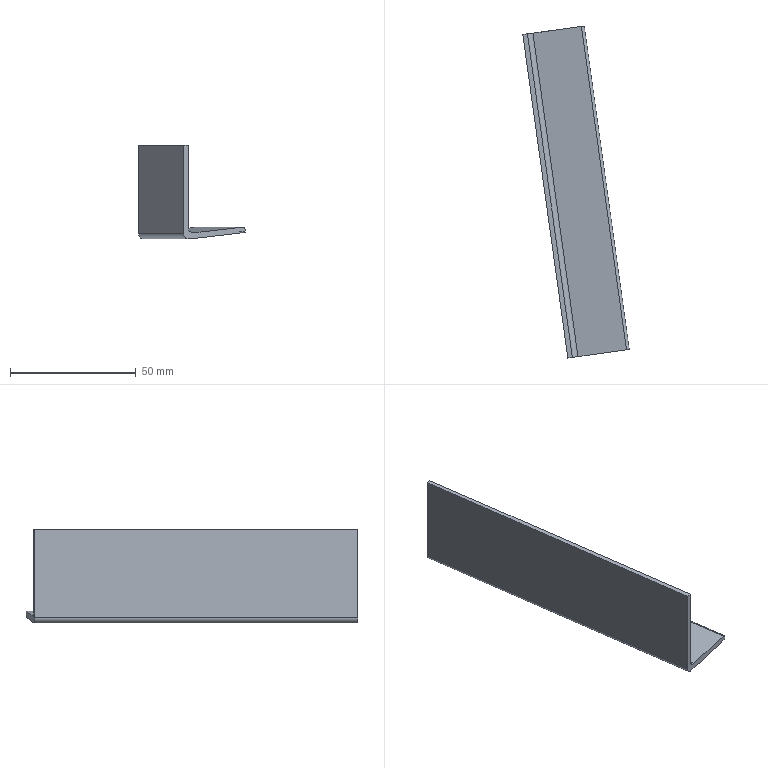Part | STEP file | 444_4 | 1 solid | 16 faces | box 42.378 x 132.163 x 37.433 mm | volume 15585 mm3 | plane 12 | cylinder 4 | commonest cylinder face diameters 4.011 x2 0.2 x1 2.007 x1
STEP:
#1=CARTESIAN_POINT('',(0.,0.,0.));
#2=DIRECTION('',(0.,0.,1.));
#3=DIRECTION('',(1.,0.,0.));
#4=AXIS2_PLACEMENT_3D('',#1,#2,#3);
#5=CARTESIAN_POINT('',(-137.211,-15.124,130.48));
#6=VERTEX_POINT('',#5);
#7=CARTESIAN_POINT('',(-119.294,-143.883,130.48));
#8=VERTEX_POINT('',#7);
#9=CARTESIAN_POINT('',(-137.211,-15.124,130.48));
#10=DIRECTION('',(0.1378,-0.9905,0.));
#11=VECTOR('',#10,1.);
#12=LINE('',#9,#11);
#13=CARTESIAN_POINT('',(-128.351,-79.517,130.48));
#14=DIRECTION('',(0.1378,-0.9905,0.));
#15=DIRECTION('',(0.9905,0.1378,0.));
#16=AXIS2_PLACEMENT_3D('',#13,#14,#15);
#17=CYLINDRICAL_SURFACE('',#16,0.09985);
#18=CARTESIAN_POINT('',(6.283,-65.));
#19=DIRECTION('',(0.,1.));
#20=VECTOR('',#19,1.);
#21=LINE('',#18,#20);
#22=(GEOMETRIC_REPRESENTATION_CONTEXT(2)PARAMETRIC_REPRESENTATION_CONTEXT()REPRESENTATION_CONTEXT('',''));
#23=DEFINITIONAL_REPRESENTATION('',(#21),#22);
#24=PCURVE('',#17,#23);
#25=CARTESIAN_POINT('',(-137.211,-15.124,131.521));
#26=DIRECTION('',(-0.9905,-0.1378,0.));
#27=DIRECTION('',(0.1378,-0.9905,0.));
#28=AXIS2_PLACEMENT_3D('',#25,#26,#27);
#29=PLANE('',#28);
#30=CARTESIAN_POINT('',(0.,-1.041));
#31=DIRECTION('',(1.,0.));
#32=VECTOR('',#31,1.);
#33=LINE('',#30,#32);
#34=(GEOMETRIC_REPRESENTATION_CONTEXT(2)PARAMETRIC_REPRESENTATION_CONTEXT()REPRESENTATION_CONTEXT('',''));
#35=DEFINITIONAL_REPRESENTATION('',(#33),#34);
#36=PCURVE('',#29,#35);
#37=SURFACE_CURVE('',#12,(#24,#36),.PCURVE_S1.);
#38=EDGE_CURVE('',#6,#8,#37,.T.);
#39=ORIENTED_EDGE('',*,*,#38,.T.);
#40=CARTESIAN_POINT('',(-119.381,-143.895,130.381));
#41=VERTEX_POINT('',#40);
#42=CARTESIAN_POINT('',(-119.392,-143.897,130.48));
#43=DIRECTION('',(-0.1378,0.9905,0.));
#44=DIRECTION('',(0.9905,0.1378,0.));
#45=AXIS2_PLACEMENT_3D('',#42,#43,#44);
#46=CIRCLE('',#45,0.09985);
#47=CARTESIAN_POINT('',(12.566,65.));
#48=DIRECTION('',(-1.,0.));
#49=VECTOR('',#48,1.);
#50=LINE('',#47,#49);
#51=(GEOMETRIC_REPRESENTATION_CONTEXT(2)PARAMETRIC_REPRESENTATION_CONTEXT()REPRESENTATION_CONTEXT('',''));
#52=DEFINITIONAL_REPRESENTATION('',(#50),#51);
#53=PCURVE('',#17,#52);
#54=CARTESIAN_POINT('',(17.376,-124.865,0.));
#55=DIRECTION('',(0.1378,-0.9905,0.));
#56=DIRECTION('',(0.9905,0.1378,0.));
#57=AXIS2_PLACEMENT_3D('',#54,#55,#56);
#58=PLANE('',#57);
#59=CARTESIAN_POINT('',(-137.986,130.48));
#60=CARTESIAN_POINT('',(-137.986,130.307));
#61=CARTESIAN_POINT('',(-138.136,130.393));
#62=CARTESIAN_POINT('',(-138.286,130.48));
#63=CARTESIAN_POINT('',(-138.136,130.566));
#64=CARTESIAN_POINT('',(-137.986,130.653));
#65=CARTESIAN_POINT('',(-137.986,130.48));
#66=(BOUNDED_CURVE()B_SPLINE_CURVE(2,(#59,#60,#61,#62,#63,#64,#65),.UNSPECIFIED.,.T.,.F.)B_SPLINE_CURVE_WITH_KNOTS((1,2,2,2,2,1),(-2.094,0.,2.094,4.189,6.283,8.378),.UNSPECIFIED.)CURVE()GEOMETRIC_REPRESENTATION_ITEM()RATIONAL_B_SPLINE_CURVE((1.,0.5,1.,0.5,1.,0.5,1.))REPRESENTATION_ITEM(''));
#67=(GEOMETRIC_REPRESENTATION_CONTEXT(2)PARAMETRIC_REPRESENTATION_CONTEXT()REPRESENTATION_CONTEXT('',''));
#68=DEFINITIONAL_REPRESENTATION('',(#66),#67);
#69=PCURVE('',#58,#68);
#70=SURFACE_CURVE('',#46,(#53,#69),.PCURVE_S1.);
#71=EDGE_CURVE('',#8,#41,#70,.T.);
#72=ORIENTED_EDGE('',*,*,#71,.T.);
#73=CARTESIAN_POINT('',(-137.299,-15.136,130.381));
#74=VERTEX_POINT('',#73);
#75=CARTESIAN_POINT('',(-119.381,-143.895,130.381));
#76=DIRECTION('',(-0.1378,0.9905,0.));
#77=VECTOR('',#76,1.);
#78=LINE('',#75,#77);
#79=CARTESIAN_POINT('',(4.827,65.));
#80=DIRECTION('',(0.,-1.));
#81=VECTOR('',#80,1.);
#82=LINE('',#79,#81);
#83=(GEOMETRIC_REPRESENTATION_CONTEXT(2)PARAMETRIC_REPRESENTATION_CONTEXT()REPRESENTATION_CONTEXT('',''));
#84=DEFINITIONAL_REPRESENTATION('',(#82),#83);
#85=PCURVE('',#17,#84);
#86=CARTESIAN_POINT('',(-137.299,-15.136,130.381));
#87=DIRECTION('',(-0.114,-0.01586,0.9934));
#88=DIRECTION('',(0.9935,0.,0.114));
#89=AXIS2_PLACEMENT_3D('',#86,#87,#88);
#90=PLANE('',#89);
#91=CARTESIAN_POINT('',(17.801,-128.775));
#92=DIRECTION('',(-0.1369,0.9906));
#93=VECTOR('',#92,1.);
#94=LINE('',#91,#93);
#95=(GEOMETRIC_REPRESENTATION_CONTEXT(2)PARAMETRIC_REPRESENTATION_CONTEXT()REPRESENTATION_CONTEXT('',''));
#96=DEFINITIONAL_REPRESENTATION('',(#94),#95);
#97=PCURVE('',#90,#96);
#98=SURFACE_CURVE('',#78,(#85,#97),.PCURVE_S1.);
#99=EDGE_CURVE('',#41,#74,#98,.T.);
#100=ORIENTED_EDGE('',*,*,#99,.T.);
#101=CARTESIAN_POINT('',(-137.31,-15.138,130.48));
#102=DIRECTION('',(0.1378,-0.9905,0.));
#103=DIRECTION('',(0.9905,0.1378,0.));
#104=AXIS2_PLACEMENT_3D('',#101,#102,#103);
#105=CIRCLE('',#104,0.09985);
#106=CARTESIAN_POINT('',(0.,-65.));
#107=DIRECTION('',(1.,0.));
#108=VECTOR('',#107,1.);
#109=LINE('',#106,#108);
#110=(GEOMETRIC_REPRESENTATION_CONTEXT(2)PARAMETRIC_REPRESENTATION_CONTEXT()REPRESENTATION_CONTEXT('',''));
#111=DEFINITIONAL_REPRESENTATION('',(#109),#110);
#112=PCURVE('',#17,#111);
#113=CARTESIAN_POINT('',(-0.5419,3.894,0.));
#114=DIRECTION('',(0.1378,-0.9905,0.));
#115=DIRECTION('',(0.9905,0.1378,0.));
#116=AXIS2_PLACEMENT_3D('',#113,#114,#115);
#117=PLANE('',#116);
#118=CARTESIAN_POINT('',(-138.086,130.48));
#119=DIRECTION('',(1.,0.));
#120=AXIS2_PLACEMENT_2D('',#118,#119);
#121=CIRCLE('',#120,0.09985);
#122=(GEOMETRIC_REPRESENTATION_CONTEXT(2)PARAMETRIC_REPRESENTATION_CONTEXT()REPRESENTATION_CONTEXT('',''));
#123=DEFINITIONAL_REPRESENTATION('',(#121),#122);
#124=PCURVE('',#117,#123);
#125=SURFACE_CURVE('',#105,(#112,#124),.PCURVE_S1.);
#126=EDGE_CURVE('',#74,#6,#125,.T.);
#127=ORIENTED_EDGE('',*,*,#126,.T.);
#128=EDGE_LOOP('',(#39,#72,#100,#127));
#129=FACE_BOUND('',#128,.T.);
#130=ADVANCED_FACE('',(#129),#17,.T.);
#131=CARTESIAN_POINT('',(-137.628,-15.182,130.342));
#132=VERTEX_POINT('',#131);
#133=CARTESIAN_POINT('',(-137.299,-15.136,130.381));
#134=DIRECTION('',(-0.9839,-0.1369,-0.1151));
#135=VECTOR('',#134,1.);
#136=LINE('',#133,#135);
#137=CARTESIAN_POINT('',(0.,0.));
#138=DIRECTION('',(-0.9906,-0.1369));
#139=VECTOR('',#138,1.);
#140=LINE('',#137,#139);
#141=(GEOMETRIC_REPRESENTATION_CONTEXT(2)PARAMETRIC_REPRESENTATION_CONTEXT()REPRESENTATION_CONTEXT('',''));
#142=DEFINITIONAL_REPRESENTATION('',(#140),#141);
#143=PCURVE('',#90,#142);
#144=CARTESIAN_POINT('',(-138.075,130.381));
#145=DIRECTION('',(-0.9934,-0.1151));
#146=VECTOR('',#145,1.);
#147=LINE('',#144,#146);
#148=(GEOMETRIC_REPRESENTATION_CONTEXT(2)PARAMETRIC_REPRESENTATION_CONTEXT()REPRESENTATION_CONTEXT('',''));
#149=DEFINITIONAL_REPRESENTATION('',(#147),#148);
#150=PCURVE('',#117,#149);
#151=SURFACE_CURVE('',#136,(#143,#150),.PCURVE_S1.);
#152=EDGE_CURVE('',#74,#132,#151,.T.);
#153=ORIENTED_EDGE('',*,*,#152,.F.);
#154=ORIENTED_EDGE('',*,*,#99,.F.);
#155=CARTESIAN_POINT('',(-119.71,-143.941,130.342));
#156=VERTEX_POINT('',#155);
#157=CARTESIAN_POINT('',(-119.71,-143.941,130.342));
#158=DIRECTION('',(0.9839,0.1369,0.1151));
#159=VECTOR('',#158,1.);
#160=LINE('',#157,#159);
#161=CARTESIAN_POINT('',(17.47,-128.821));
#162=DIRECTION('',(0.9906,0.1369));
#163=VECTOR('',#162,1.);
#164=LINE('',#161,#163);
#165=(GEOMETRIC_REPRESENTATION_CONTEXT(2)PARAMETRIC_REPRESENTATION_CONTEXT()REPRESENTATION_CONTEXT('',''));
#166=DEFINITIONAL_REPRESENTATION('',(#164),#165);
#167=PCURVE('',#90,#166);
#168=CARTESIAN_POINT('',(-138.407,130.342));
#169=DIRECTION('',(0.9934,0.1151));
#170=VECTOR('',#169,1.);
#171=LINE('',#168,#170);
#172=(GEOMETRIC_REPRESENTATION_CONTEXT(2)PARAMETRIC_REPRESENTATION_CONTEXT()REPRESENTATION_CONTEXT('',''));
#173=DEFINITIONAL_REPRESENTATION('',(#171),#172);
#174=PCURVE('',#58,#173);
#175=SURFACE_CURVE('',#160,(#167,#174),.PCURVE_S1.);
#176=EDGE_CURVE('',#156,#41,#175,.T.);
#177=ORIENTED_EDGE('',*,*,#176,.F.);
#178=CARTESIAN_POINT('',(-137.628,-15.182,130.342));
#179=DIRECTION('',(-0.1378,0.9905,0.));
#180=VECTOR('',#179,1.);
#181=LINE('',#178,#180);
#182=CARTESIAN_POINT('',(-0.3313,-0.04579));
#183=DIRECTION('',(-0.1369,0.9906));
#184=VECTOR('',#183,1.);
#185=LINE('',#182,#184);
#186=(GEOMETRIC_REPRESENTATION_CONTEXT(2)PARAMETRIC_REPRESENTATION_CONTEXT()REPRESENTATION_CONTEXT('',''));
#187=DEFINITIONAL_REPRESENTATION('',(#185),#186);
#188=PCURVE('',#90,#187);
#189=CARTESIAN_POINT('',(-137.628,-15.182,130.342));
#190=DIRECTION('',(0.9905,0.1378,-0.000000003));
#191=DIRECTION('',(-0.1378,0.9905,0.));
#192=AXIS2_PLACEMENT_3D('',#189,#190,#191);
#193=PLANE('',#192);
#194=CARTESIAN_POINT('',(0.,0.));
#195=DIRECTION('',(1.,0.));
#196=VECTOR('',#195,1.);
#197=LINE('',#194,#196);
#198=(GEOMETRIC_REPRESENTATION_CONTEXT(2)PARAMETRIC_REPRESENTATION_CONTEXT()REPRESENTATION_CONTEXT('',''));
#199=DEFINITIONAL_REPRESENTATION('',(#197),#198);
#200=PCURVE('',#193,#199);
#201=SURFACE_CURVE('',#181,(#188,#200),.PCURVE_S1.);
#202=EDGE_CURVE('',#156,#132,#201,.T.);
#203=ORIENTED_EDGE('',*,*,#202,.T.);
#204=EDGE_LOOP('',(#153,#154,#177,#203));
#205=FACE_BOUND('',#204,.T.);
#206=ADVANCED_FACE('',(#205),#90,.F.);
#207=CARTESIAN_POINT('',(-137.211,-15.124,131.521));
#208=VERTEX_POINT('',#207);
#209=CARTESIAN_POINT('',(-137.211,-15.124,131.521));
#210=DIRECTION('',(0.,0.,-1.));
#211=VECTOR('',#210,1.);
#212=LINE('',#209,#211);
#213=CARTESIAN_POINT('',(0.,0.));
#214=DIRECTION('',(0.,-1.));
#215=VECTOR('',#214,1.);
#216=LINE('',#213,#215);
#217=(GEOMETRIC_REPRESENTATION_CONTEXT(2)PARAMETRIC_REPRESENTATION_CONTEXT()REPRESENTATION_CONTEXT('',''));
#218=DEFINITIONAL_REPRESENTATION('',(#216),#217);
#219=PCURVE('',#29,#218);
#220=CARTESIAN_POINT('',(-137.986,131.521));
#221=DIRECTION('',(0.,-1.));
#222=VECTOR('',#221,1.);
#223=LINE('',#220,#222);
#224=(GEOMETRIC_REPRESENTATION_CONTEXT(2)PARAMETRIC_REPRESENTATION_CONTEXT()REPRESENTATION_CONTEXT('',''));
#225=DEFINITIONAL_REPRESENTATION('',(#223),#224);
#226=PCURVE('',#117,#225);
#227=SURFACE_CURVE('',#212,(#219,#226),.PCURVE_S1.);
#228=EDGE_CURVE('',#208,#6,#227,.T.);
#229=ORIENTED_EDGE('',*,*,#228,.F.);
#230=CARTESIAN_POINT('',(-119.294,-143.883,131.521));
#231=VERTEX_POINT('',#230);
#232=CARTESIAN_POINT('',(-128.252,-79.504,131.521));
#233=DIRECTION('',(-0.1378,0.9905,0.));
#234=VECTOR('',#233,1.);
#235=LINE('',#232,#234);
#236=CARTESIAN_POINT('',(65.,0.));
#237=DIRECTION('',(-1.,0.));
#238=VECTOR('',#237,1.);
#239=LINE('',#236,#238);
#240=(GEOMETRIC_REPRESENTATION_CONTEXT(2)PARAMETRIC_REPRESENTATION_CONTEXT()REPRESENTATION_CONTEXT('',''));
#241=DEFINITIONAL_REPRESENTATION('',(#239),#240);
#242=PCURVE('',#29,#241);
#243=CARTESIAN_POINT('',(-129.246,-79.642,131.52));
#244=DIRECTION('',(0.1378,-0.9905,0.));
#245=DIRECTION('',(0.9905,0.1378,0.));
#246=AXIS2_PLACEMENT_3D('',#243,#244,#245);
#247=CYLINDRICAL_SURFACE('',#246,1.004);
#248=CARTESIAN_POINT('',(0.0006999,0.));
#249=DIRECTION('',(0.,-1.));
#250=VECTOR('',#249,1.);
#251=LINE('',#248,#250);
#252=(GEOMETRIC_REPRESENTATION_CONTEXT(2)PARAMETRIC_REPRESENTATION_CONTEXT()REPRESENTATION_CONTEXT('',''));
#253=DEFINITIONAL_REPRESENTATION('',(#251),#252);
#254=PCURVE('',#247,#253);
#255=SURFACE_CURVE('',#235,(#242,#254),.PCURVE_S1.);
#256=EDGE_CURVE('',#231,#208,#255,.T.);
#257=ORIENTED_EDGE('',*,*,#256,.F.);
#258=CARTESIAN_POINT('',(-119.294,-143.883,131.521));
#259=DIRECTION('',(0.,0.,1.));
#260=VECTOR('',#259,1.);
#261=LINE('',#258,#260);
#262=CARTESIAN_POINT('',(130.,0.));
#263=DIRECTION('',(0.,1.));
#264=VECTOR('',#263,1.);
#265=LINE('',#262,#264);
#266=(GEOMETRIC_REPRESENTATION_CONTEXT(2)PARAMETRIC_REPRESENTATION_CONTEXT()REPRESENTATION_CONTEXT('',''));
#267=DEFINITIONAL_REPRESENTATION('',(#265),#266);
#268=PCURVE('',#29,#267);
#269=CARTESIAN_POINT('',(-137.986,131.521));
#270=DIRECTION('',(0.,1.));
#271=VECTOR('',#270,1.);
#272=LINE('',#269,#271);
#273=(GEOMETRIC_REPRESENTATION_CONTEXT(2)PARAMETRIC_REPRESENTATION_CONTEXT()REPRESENTATION_CONTEXT('',''));
#274=DEFINITIONAL_REPRESENTATION('',(#272),#273);
#275=PCURVE('',#58,#274);
#276=SURFACE_CURVE('',#261,(#268,#275),.PCURVE_S1.);
#277=EDGE_CURVE('',#8,#231,#276,.T.);
#278=ORIENTED_EDGE('',*,*,#277,.F.);
#279=ORIENTED_EDGE('',*,*,#38,.F.);
#280=EDGE_LOOP('',(#229,#257,#278,#279));
#281=FACE_BOUND('',#280,.T.);
#282=ADVANCED_FACE('',(#281),#29,.F.);
#283=CARTESIAN_POINT('',(-137.628,-15.182,130.687));
#284=VERTEX_POINT('',#283);
#285=CARTESIAN_POINT('',(-137.628,-15.182,130.342));
#286=DIRECTION('',(0.000000003,0.,1.));
#287=VECTOR('',#286,1.);
#288=LINE('',#285,#287);
#289=CARTESIAN_POINT('',(0.,0.));
#290=DIRECTION('',(0.,1.));
#291=VECTOR('',#290,1.);
#292=LINE('',#289,#291);
#293=(GEOMETRIC_REPRESENTATION_CONTEXT(2)PARAMETRIC_REPRESENTATION_CONTEXT()REPRESENTATION_CONTEXT('',''));
#294=DEFINITIONAL_REPRESENTATION('',(#292),#293);
#295=PCURVE('',#193,#294);
#296=CARTESIAN_POINT('',(-138.407,130.342));
#297=DIRECTION('',(0.000000003,1.));
#298=VECTOR('',#297,1.);
#299=LINE('',#296,#298);
#300=(GEOMETRIC_REPRESENTATION_CONTEXT(2)PARAMETRIC_REPRESENTATION_CONTEXT()REPRESENTATION_CONTEXT('',''));
#301=DEFINITIONAL_REPRESENTATION('',(#299),#300);
#302=PCURVE('',#117,#301);
#303=SURFACE_CURVE('',#288,(#295,#302),.PCURVE_S1.);
#304=EDGE_CURVE('',#132,#284,#303,.T.);
#305=ORIENTED_EDGE('',*,*,#304,.F.);
#306=ORIENTED_EDGE('',*,*,#202,.F.);
#307=CARTESIAN_POINT('',(-119.71,-143.941,130.687));
#308=VERTEX_POINT('',#307);
#309=CARTESIAN_POINT('',(-119.71,-143.941,130.342));
#310=DIRECTION('',(-0.000000003,0.,-1.));
#311=VECTOR('',#310,1.);
#312=LINE('',#309,#311);
#313=CARTESIAN_POINT('',(-130.,0.));
#314=DIRECTION('',(0.,-1.));
#315=VECTOR('',#314,1.);
#316=LINE('',#313,#315);
#317=(GEOMETRIC_REPRESENTATION_CONTEXT(2)PARAMETRIC_REPRESENTATION_CONTEXT()REPRESENTATION_CONTEXT('',''));
#318=DEFINITIONAL_REPRESENTATION('',(#316),#317);
#319=PCURVE('',#193,#318);
#320=CARTESIAN_POINT('',(-138.407,130.342));
#321=DIRECTION('',(-0.000000003,-1.));
#322=VECTOR('',#321,1.);
#323=LINE('',#320,#322);
#324=(GEOMETRIC_REPRESENTATION_CONTEXT(2)PARAMETRIC_REPRESENTATION_CONTEXT()REPRESENTATION_CONTEXT('',''));
#325=DEFINITIONAL_REPRESENTATION('',(#323),#324);
#326=PCURVE('',#58,#325);
#327=SURFACE_CURVE('',#312,(#319,#326),.PCURVE_S1.);
#328=EDGE_CURVE('',#308,#156,#327,.T.);
#329=ORIENTED_EDGE('',*,*,#328,.F.);
#330=CARTESIAN_POINT('',(-119.71,-143.941,130.687));
#331=DIRECTION('',(-0.1378,0.9905,0.));
#332=VECTOR('',#331,1.);
#333=LINE('',#330,#332);
#334=CARTESIAN_POINT('',(-130.,0.3449));
#335=DIRECTION('',(1.,0.));
#336=VECTOR('',#335,1.);
#337=LINE('',#334,#336);
#338=(GEOMETRIC_REPRESENTATION_CONTEXT(2)PARAMETRIC_REPRESENTATION_CONTEXT()REPRESENTATION_CONTEXT('',''));
#339=DEFINITIONAL_REPRESENTATION('',(#337),#338);
#340=PCURVE('',#193,#339);
#341=CARTESIAN_POINT('',(-137.628,-15.182,130.687));
#342=DIRECTION('',(0.0002938,0.00004088,1.));
#343=DIRECTION('',(1.,0.,-0.0002938));
#344=AXIS2_PLACEMENT_3D('',#341,#342,#343);
#345=PLANE('',#344);
#346=CARTESIAN_POINT('',(17.918,-128.759));
#347=DIRECTION('',(-0.1378,0.9905));
#348=VECTOR('',#347,1.);
#349=LINE('',#346,#348);
#350=(GEOMETRIC_REPRESENTATION_CONTEXT(2)PARAMETRIC_REPRESENTATION_CONTEXT()REPRESENTATION_CONTEXT('',''));
#351=DEFINITIONAL_REPRESENTATION('',(#349),#350);
#352=PCURVE('',#345,#351);
#353=SURFACE_CURVE('',#333,(#340,#352),.PCURVE_S1.);
#354=EDGE_CURVE('',#308,#284,#353,.T.);
#355=ORIENTED_EDGE('',*,*,#354,.T.);
#356=EDGE_LOOP('',(#305,#306,#329,#355));
#357=FACE_BOUND('',#356,.T.);
#358=ADVANCED_FACE('',(#357),#193,.F.);
#359=CARTESIAN_POINT('',(-138.319,-15.278,132.517));
#360=VERTEX_POINT('',#359);
#361=CARTESIAN_POINT('',(-120.402,-144.037,132.517));
#362=VERTEX_POINT('',#361);
#363=CARTESIAN_POINT('',(-138.319,-15.278,132.517));
#364=DIRECTION('',(0.1378,-0.9905,0.));
#365=VECTOR('',#364,1.);
#366=LINE('',#363,#365);
#367=CARTESIAN_POINT('',(1.686,-65.));
#368=DIRECTION('',(0.,1.));
#369=VECTOR('',#368,1.);
#370=LINE('',#367,#369);
#371=(GEOMETRIC_REPRESENTATION_CONTEXT(2)PARAMETRIC_REPRESENTATION_CONTEXT()REPRESENTATION_CONTEXT('',''));
#372=DEFINITIONAL_REPRESENTATION('',(#370),#371);
#373=PCURVE('',#247,#372);
#374=CARTESIAN_POINT('',(-157.626,-17.965,130.259));
#375=DIRECTION('',(0.114,0.01586,-0.9934));
#376=DIRECTION('',(-0.9935,0.,-0.114));
#377=AXIS2_PLACEMENT_3D('',#374,#375,#376);
#378=PLANE('',#377);
#379=CARTESIAN_POINT('',(-19.438,2.687));
#380=DIRECTION('',(-0.1369,-0.9906));
#381=VECTOR('',#380,1.);
#382=LINE('',#379,#381);
#383=(GEOMETRIC_REPRESENTATION_CONTEXT(2)PARAMETRIC_REPRESENTATION_CONTEXT()REPRESENTATION_CONTEXT('',''));
#384=DEFINITIONAL_REPRESENTATION('',(#382),#383);
#385=PCURVE('',#378,#384);
#386=SURFACE_CURVE('',#366,(#373,#385),.PCURVE_S1.);
#387=EDGE_CURVE('',#360,#362,#386,.T.);
#388=ORIENTED_EDGE('',*,*,#387,.T.);
#389=CARTESIAN_POINT('',(-120.288,-144.022,131.52));
#390=DIRECTION('',(-0.1378,0.9905,0.));
#391=DIRECTION('',(0.9905,0.1378,0.));
#392=AXIS2_PLACEMENT_3D('',#389,#390,#391);
#393=CIRCLE('',#392,1.004);
#394=CARTESIAN_POINT('',(6.283,65.));
#395=DIRECTION('',(-1.,0.));
#396=VECTOR('',#395,1.);
#397=LINE('',#394,#396);
#398=(GEOMETRIC_REPRESENTATION_CONTEXT(2)PARAMETRIC_REPRESENTATION_CONTEXT()REPRESENTATION_CONTEXT('',''));
#399=DEFINITIONAL_REPRESENTATION('',(#397),#398);
#400=PCURVE('',#247,#399);
#401=CARTESIAN_POINT('',(-137.986,131.52));
#402=CARTESIAN_POINT('',(-137.986,129.782));
#403=CARTESIAN_POINT('',(-139.492,130.651));
#404=CARTESIAN_POINT('',(-140.997,131.52));
#405=CARTESIAN_POINT('',(-139.492,132.39));
#406=CARTESIAN_POINT('',(-137.986,133.259));
#407=CARTESIAN_POINT('',(-137.986,131.52));
#408=(BOUNDED_CURVE()B_SPLINE_CURVE(2,(#401,#402,#403,#404,#405,#406,#407),.UNSPECIFIED.,.T.,.F.)B_SPLINE_CURVE_WITH_KNOTS((1,2,2,2,2,1),(-2.094,0.,2.094,4.189,6.283,8.378),.UNSPECIFIED.)CURVE()GEOMETRIC_REPRESENTATION_ITEM()RATIONAL_B_SPLINE_CURVE((1.,0.5,1.,0.5,1.,0.5,1.))REPRESENTATION_ITEM(''));
#409=(GEOMETRIC_REPRESENTATION_CONTEXT(2)PARAMETRIC_REPRESENTATION_CONTEXT()REPRESENTATION_CONTEXT('',''));
#410=DEFINITIONAL_REPRESENTATION('',(#408),#409);
#411=PCURVE('',#58,#410);
#412=SURFACE_CURVE('',#393,(#400,#411),.PCURVE_S1.);
#413=EDGE_CURVE('',#362,#231,#412,.T.);
#414=ORIENTED_EDGE('',*,*,#413,.T.);
#415=ORIENTED_EDGE('',*,*,#256,.T.);
#416=CARTESIAN_POINT('',(-138.205,-15.262,131.52));
#417=DIRECTION('',(0.1378,-0.9905,0.));
#418=DIRECTION('',(0.9905,0.1378,0.));
#419=AXIS2_PLACEMENT_3D('',#416,#417,#418);
#420=CIRCLE('',#419,1.004);
#421=CARTESIAN_POINT('',(0.,-65.));
#422=DIRECTION('',(1.,0.));
#423=VECTOR('',#422,1.);
#424=LINE('',#421,#423);
#425=(GEOMETRIC_REPRESENTATION_CONTEXT(2)PARAMETRIC_REPRESENTATION_CONTEXT()REPRESENTATION_CONTEXT('',''));
#426=DEFINITIONAL_REPRESENTATION('',(#424),#425);
#427=PCURVE('',#247,#426);
#428=CARTESIAN_POINT('',(-138.99,131.52));
#429=DIRECTION('',(1.,0.));
#430=AXIS2_PLACEMENT_2D('',#428,#429);
#431=CIRCLE('',#430,1.004);
#432=(GEOMETRIC_REPRESENTATION_CONTEXT(2)PARAMETRIC_REPRESENTATION_CONTEXT()REPRESENTATION_CONTEXT('',''));
#433=DEFINITIONAL_REPRESENTATION('',(#431),#432);
#434=PCURVE('',#117,#433);
#435=SURFACE_CURVE('',#420,(#427,#434),.PCURVE_S1.);
#436=EDGE_CURVE('',#208,#360,#435,.T.);
#437=ORIENTED_EDGE('',*,*,#436,.T.);
#438=EDGE_LOOP('',(#388,#414,#415,#437));
#439=FACE_BOUND('',#438,.T.);
#440=ADVANCED_FACE('',(#439),#247,.T.);
#441=CARTESIAN_POINT('',(-139.46,-15.437,130.688));
#442=VERTEX_POINT('',#441);
#443=CARTESIAN_POINT('',(-139.46,-15.437,130.128));
#444=VERTEX_POINT('',#443);
#445=CARTESIAN_POINT('',(-139.46,-15.437,130.688));
#446=DIRECTION('',(0.,0.,-1.));
#447=VECTOR('',#446,1.);
#448=LINE('',#445,#447);
#449=CARTESIAN_POINT('',(-139.46,-15.437,130.688));
#450=DIRECTION('',(-0.9905,-0.1378,0.));
#451=DIRECTION('',(0.1378,-0.9905,0.));
#452=AXIS2_PLACEMENT_3D('',#449,#450,#451);
#453=PLANE('',#452);
#454=CARTESIAN_POINT('',(0.,0.));
#455=DIRECTION('',(0.,-1.));
#456=VECTOR('',#455,1.);
#457=LINE('',#454,#456);
#458=(GEOMETRIC_REPRESENTATION_CONTEXT(2)PARAMETRIC_REPRESENTATION_CONTEXT()REPRESENTATION_CONTEXT('',''));
#459=DEFINITIONAL_REPRESENTATION('',(#457),#458);
#460=PCURVE('',#453,#459);
#461=CARTESIAN_POINT('',(-140.256,130.688));
#462=DIRECTION('',(0.,-1.));
#463=VECTOR('',#462,1.);
#464=LINE('',#461,#463);
#465=(GEOMETRIC_REPRESENTATION_CONTEXT(2)PARAMETRIC_REPRESENTATION_CONTEXT()REPRESENTATION_CONTEXT('',''));
#466=DEFINITIONAL_REPRESENTATION('',(#464),#465);
#467=PCURVE('',#117,#466);
#468=SURFACE_CURVE('',#448,(#460,#467),.PCURVE_S1.);
#469=EDGE_CURVE('',#442,#444,#468,.T.);
#470=ORIENTED_EDGE('',*,*,#469,.F.);
#471=CARTESIAN_POINT('',(-121.542,-144.196,130.688));
#472=VERTEX_POINT('',#471);
#473=CARTESIAN_POINT('',(-139.46,-15.437,130.688));
#474=DIRECTION('',(0.1378,-0.9905,0.));
#475=VECTOR('',#474,1.);
#476=LINE('',#473,#475);
#477=CARTESIAN_POINT('',(0.,0.));
#478=DIRECTION('',(1.,0.));
#479=VECTOR('',#478,1.);
#480=LINE('',#477,#479);
#481=(GEOMETRIC_REPRESENTATION_CONTEXT(2)PARAMETRIC_REPRESENTATION_CONTEXT()REPRESENTATION_CONTEXT('',''));
#482=DEFINITIONAL_REPRESENTATION('',(#480),#481);
#483=PCURVE('',#453,#482);
#484=CARTESIAN_POINT('',(-1.832,-0.2549));
#485=DIRECTION('',(0.1378,-0.9905));
#486=VECTOR('',#485,1.);
#487=LINE('',#484,#486);
#488=(GEOMETRIC_REPRESENTATION_CONTEXT(2)PARAMETRIC_REPRESENTATION_CONTEXT()REPRESENTATION_CONTEXT('',''));
#489=DEFINITIONAL_REPRESENTATION('',(#487),#488);
#490=PCURVE('',#345,#489);
#491=SURFACE_CURVE('',#476,(#483,#490),.PCURVE_S1.);
#492=EDGE_CURVE('',#442,#472,#491,.T.);
#493=ORIENTED_EDGE('',*,*,#492,.T.);
#494=CARTESIAN_POINT('',(-121.542,-144.196,130.128));
#495=VERTEX_POINT('',#494);
#496=CARTESIAN_POINT('',(-121.542,-144.196,130.688));
#497=DIRECTION('',(0.,0.,1.));
#498=VECTOR('',#497,1.);
#499=LINE('',#496,#498);
#500=CARTESIAN_POINT('',(130.,0.));
#501=DIRECTION('',(0.,1.));
#502=VECTOR('',#501,1.);
#503=LINE('',#500,#502);
#504=(GEOMETRIC_REPRESENTATION_CONTEXT(2)PARAMETRIC_REPRESENTATION_CONTEXT()REPRESENTATION_CONTEXT('',''));
#505=DEFINITIONAL_REPRESENTATION('',(#503),#504);
#506=PCURVE('',#453,#505);
#507=CARTESIAN_POINT('',(-140.256,130.688));
#508=DIRECTION('',(0.,1.));
#509=VECTOR('',#508,1.);
#510=LINE('',#507,#509);
#511=(GEOMETRIC_REPRESENTATION_CONTEXT(2)PARAMETRIC_REPRESENTATION_CONTEXT()REPRESENTATION_CONTEXT('',''));
#512=DEFINITIONAL_REPRESENTATION('',(#510),#511);
#513=PCURVE('',#58,#512);
#514=SURFACE_CURVE('',#499,(#506,#513),.PCURVE_S1.);
#515=EDGE_CURVE('',#495,#472,#514,.T.);
#516=ORIENTED_EDGE('',*,*,#515,.F.);
#517=CARTESIAN_POINT('',(-121.542,-144.196,130.128));
#518=DIRECTION('',(-0.1378,0.9905,0.));
#519=VECTOR('',#518,1.);
#520=LINE('',#517,#519);
#521=CARTESIAN_POINT('',(130.,-0.5598));
#522=DIRECTION('',(-1.,0.));
#523=VECTOR('',#522,1.);
#524=LINE('',#521,#523);
#525=(GEOMETRIC_REPRESENTATION_CONTEXT(2)PARAMETRIC_REPRESENTATION_CONTEXT()REPRESENTATION_CONTEXT('',''));
#526=DEFINITIONAL_REPRESENTATION('',(#524),#525);
#527=PCURVE('',#453,#526);
#528=CARTESIAN_POINT('',(-137.299,-15.136,130.381));
#529=DIRECTION('',(-0.114,-0.01586,0.9934));
#530=DIRECTION('',(0.9935,0.,0.114));
#531=AXIS2_PLACEMENT_3D('',#528,#529,#530);
#532=PLANE('',#531);
#533=CARTESIAN_POINT('',(15.625,-129.076));
#534=DIRECTION('',(-0.1369,0.9906));
#535=VECTOR('',#534,1.);
#536=LINE('',#533,#535);
#537=(GEOMETRIC_REPRESENTATION_CONTEXT(2)PARAMETRIC_REPRESENTATION_CONTEXT()REPRESENTATION_CONTEXT('',''));
#538=DEFINITIONAL_REPRESENTATION('',(#536),#537);
#539=PCURVE('',#532,#538);
#540=SURFACE_CURVE('',#520,(#527,#539),.PCURVE_S1.);
#541=EDGE_CURVE('',#495,#444,#540,.T.);
#542=ORIENTED_EDGE('',*,*,#541,.T.);
#543=EDGE_LOOP('',(#470,#493,#516,#542));
#544=FACE_BOUND('',#543,.T.);
#545=ADVANCED_FACE('',(#544),#453,.F.);
#546=CARTESIAN_POINT('',(-139.46,-15.437,130.688));
#547=DIRECTION('',(0.9905,0.1378,-0.0002966));
#548=VECTOR('',#547,1.);
#549=LINE('',#546,#548);
#550=CARTESIAN_POINT('',(-1.832,-0.2549));
#551=DIRECTION('',(0.9905,0.1378));
#552=VECTOR('',#551,1.);
#553=LINE('',#550,#552);
#554=(GEOMETRIC_REPRESENTATION_CONTEXT(2)PARAMETRIC_REPRESENTATION_CONTEXT()REPRESENTATION_CONTEXT('',''));
#555=DEFINITIONAL_REPRESENTATION('',(#553),#554);
#556=PCURVE('',#345,#555);
#557=CARTESIAN_POINT('',(-140.256,130.688));
#558=DIRECTION('',(1.,-0.0002966));
#559=VECTOR('',#558,1.);
#560=LINE('',#557,#559);
#561=(GEOMETRIC_REPRESENTATION_CONTEXT(2)PARAMETRIC_REPRESENTATION_CONTEXT()REPRESENTATION_CONTEXT('',''));
#562=DEFINITIONAL_REPRESENTATION('',(#560),#561);
#563=PCURVE('',#117,#562);
#564=SURFACE_CURVE('',#549,(#556,#563),.PCURVE_S1.);
#565=EDGE_CURVE('',#442,#284,#564,.T.);
#566=ORIENTED_EDGE('',*,*,#565,.T.);
#567=ORIENTED_EDGE('',*,*,#354,.F.);
#568=CARTESIAN_POINT('',(-121.542,-144.196,130.688));
#569=DIRECTION('',(0.9905,0.1378,-0.0002966));
#570=VECTOR('',#569,1.);
#571=LINE('',#568,#570);
#572=CARTESIAN_POINT('',(16.086,-129.014));
#573=DIRECTION('',(0.9905,0.1378));
#574=VECTOR('',#573,1.);
#575=LINE('',#572,#574);
#576=(GEOMETRIC_REPRESENTATION_CONTEXT(2)PARAMETRIC_REPRESENTATION_CONTEXT()REPRESENTATION_CONTEXT('',''));
#577=DEFINITIONAL_REPRESENTATION('',(#575),#576);
#578=PCURVE('',#345,#577);
#579=CARTESIAN_POINT('',(-140.256,130.688));
#580=DIRECTION('',(1.,-0.0002966));
#581=VECTOR('',#580,1.);
#582=LINE('',#579,#581);
#583=(GEOMETRIC_REPRESENTATION_CONTEXT(2)PARAMETRIC_REPRESENTATION_CONTEXT()REPRESENTATION_CONTEXT('',''));
#584=DEFINITIONAL_REPRESENTATION('',(#582),#583);
#585=PCURVE('',#58,#584);
#586=SURFACE_CURVE('',#571,(#578,#585),.PCURVE_S1.);
#587=EDGE_CURVE('',#472,#308,#586,.T.);
#588=ORIENTED_EDGE('',*,*,#587,.F.);
#589=ORIENTED_EDGE('',*,*,#492,.F.);
#590=EDGE_LOOP('',(#566,#567,#588,#589));
#591=FACE_BOUND('',#590,.T.);
#592=ADVANCED_FACE('',(#591),#345,.F.);
#593=CARTESIAN_POINT('',(-157.626,-17.965,130.259));
#594=VERTEX_POINT('',#593);
#595=CARTESIAN_POINT('',(-138.319,-15.278,132.517));
#596=DIRECTION('',(-0.9839,-0.1369,-0.1151));
#597=VECTOR('',#596,1.);
#598=LINE('',#595,#597);
#599=CARTESIAN_POINT('',(-19.438,2.687));
#600=DIRECTION('',(0.9906,-0.1369));
#601=VECTOR('',#600,1.);
#602=LINE('',#599,#601);
#603=(GEOMETRIC_REPRESENTATION_CONTEXT(2)PARAMETRIC_REPRESENTATION_CONTEXT()REPRESENTATION_CONTEXT('',''));
#604=DEFINITIONAL_REPRESENTATION('',(#602),#603);
#605=PCURVE('',#378,#604);
#606=CARTESIAN_POINT('',(-139.105,132.517));
#607=DIRECTION('',(-0.9934,-0.1151));
#608=VECTOR('',#607,1.);
#609=LINE('',#606,#608);
#610=(GEOMETRIC_REPRESENTATION_CONTEXT(2)PARAMETRIC_REPRESENTATION_CONTEXT()REPRESENTATION_CONTEXT('',''));
#611=DEFINITIONAL_REPRESENTATION('',(#609),#610);
#612=PCURVE('',#117,#611);
#613=SURFACE_CURVE('',#598,(#605,#612),.PCURVE_S1.);
#614=EDGE_CURVE('',#360,#594,#613,.T.);
#615=ORIENTED_EDGE('',*,*,#614,.T.);
#616=CARTESIAN_POINT('',(-139.708,-146.724,130.259));
#617=VERTEX_POINT('',#616);
#618=CARTESIAN_POINT('',(-148.667,-82.344,130.259));
#619=DIRECTION('',(0.1378,-0.9905,0.));
#620=VECTOR('',#619,1.);
#621=LINE('',#618,#620);
#622=CARTESIAN_POINT('',(-8.9,-64.388));
#623=DIRECTION('',(-0.1369,-0.9906));
#624=VECTOR('',#623,1.);
#625=LINE('',#622,#624);
#626=(GEOMETRIC_REPRESENTATION_CONTEXT(2)PARAMETRIC_REPRESENTATION_CONTEXT()REPRESENTATION_CONTEXT('',''));
#627=DEFINITIONAL_REPRESENTATION('',(#625),#626);
#628=PCURVE('',#378,#627);
#629=CARTESIAN_POINT('',(-148.895,-82.376,132.251));
#630=DIRECTION('',(0.1378,-0.9905,0.));
#631=DIRECTION('',(0.9905,0.1378,0.));
#632=AXIS2_PLACEMENT_3D('',#629,#630,#631);
#633=CYLINDRICAL_SURFACE('',#632,2.005);
#634=CARTESIAN_POINT('',(4.828,0.));
#635=DIRECTION('',(0.,1.));
#636=VECTOR('',#635,1.);
#637=LINE('',#634,#636);
#638=(GEOMETRIC_REPRESENTATION_CONTEXT(2)PARAMETRIC_REPRESENTATION_CONTEXT()REPRESENTATION_CONTEXT('',''));
#639=DEFINITIONAL_REPRESENTATION('',(#637),#638);
#640=PCURVE('',#633,#639);
#641=SURFACE_CURVE('',#621,(#628,#640),.PCURVE_S1.);
#642=EDGE_CURVE('',#594,#617,#641,.T.);
#643=ORIENTED_EDGE('',*,*,#642,.T.);
#644=CARTESIAN_POINT('',(-120.402,-144.037,132.517));
#645=DIRECTION('',(-0.9839,-0.1369,-0.1151));
#646=VECTOR('',#645,1.);
#647=LINE('',#644,#646);
#648=CARTESIAN_POINT('',(-37.239,-126.089));
#649=DIRECTION('',(0.9906,-0.1369));
#650=VECTOR('',#649,1.);
#651=LINE('',#648,#650);
#652=(GEOMETRIC_REPRESENTATION_CONTEXT(2)PARAMETRIC_REPRESENTATION_CONTEXT()REPRESENTATION_CONTEXT('',''));
#653=DEFINITIONAL_REPRESENTATION('',(#651),#652);
#654=PCURVE('',#378,#653);
#655=CARTESIAN_POINT('',(-139.105,132.517));
#656=DIRECTION('',(-0.9934,-0.1151));
#657=VECTOR('',#656,1.);
#658=LINE('',#655,#657);
#659=(GEOMETRIC_REPRESENTATION_CONTEXT(2)PARAMETRIC_REPRESENTATION_CONTEXT()REPRESENTATION_CONTEXT('',''));
#660=DEFINITIONAL_REPRESENTATION('',(#658),#659);
#661=PCURVE('',#58,#660);
#662=SURFACE_CURVE('',#647,(#654,#661),.PCURVE_S1.);
#663=EDGE_CURVE('',#362,#617,#662,.T.);
#664=ORIENTED_EDGE('',*,*,#663,.F.);
#665=ORIENTED_EDGE('',*,*,#387,.F.);
#666=EDGE_LOOP('',(#615,#643,#664,#665));
#667=FACE_BOUND('',#666,.T.);
#668=ADVANCED_FACE('',(#667),#378,.F.);
#669=ORIENTED_EDGE('',*,*,#642,.T.);
#670=CARTESIAN_POINT('',(-141.923,-147.032,132.25));
#671=VERTEX_POINT('',#670);
#672=CARTESIAN_POINT('',(-139.936,-146.756,132.251));
#673=DIRECTION('',(-0.1378,0.9905,0.));
#674=DIRECTION('',(0.9905,0.1378,0.));
#675=AXIS2_PLACEMENT_3D('',#672,#673,#674);
#676=CIRCLE('',#675,2.005);
#677=CARTESIAN_POINT('',(6.283,65.));
#678=DIRECTION('',(-1.,0.));
#679=VECTOR('',#678,1.);
#680=LINE('',#677,#679);
#681=(GEOMETRIC_REPRESENTATION_CONTEXT(2)PARAMETRIC_REPRESENTATION_CONTEXT()REPRESENTATION_CONTEXT('',''));
#682=DEFINITIONAL_REPRESENTATION('',(#680),#681);
#683=PCURVE('',#633,#682);
#684=CARTESIAN_POINT('',(-156.822,132.251));
#685=CARTESIAN_POINT('',(-156.822,128.778));
#686=CARTESIAN_POINT('',(-159.831,130.514));
#687=CARTESIAN_POINT('',(-162.839,132.251));
#688=CARTESIAN_POINT('',(-159.831,133.988));
#689=CARTESIAN_POINT('',(-156.822,135.725));
#690=CARTESIAN_POINT('',(-156.822,132.251));
#691=(BOUNDED_CURVE()B_SPLINE_CURVE(2,(#684,#685,#686,#687,#688,#689,#690),.UNSPECIFIED.,.T.,.F.)B_SPLINE_CURVE_WITH_KNOTS((1,2,2,2,2,1),(-2.094,0.,2.094,4.189,6.283,8.378),.UNSPECIFIED.)CURVE()GEOMETRIC_REPRESENTATION_ITEM()RATIONAL_B_SPLINE_CURVE((1.,0.5,1.,0.5,1.,0.5,1.))REPRESENTATION_ITEM(''));
#692=(GEOMETRIC_REPRESENTATION_CONTEXT(2)PARAMETRIC_REPRESENTATION_CONTEXT()REPRESENTATION_CONTEXT('',''));
#693=DEFINITIONAL_REPRESENTATION('',(#691),#692);
#694=PCURVE('',#58,#693);
#695=SURFACE_CURVE('',#676,(#683,#694),.PCURVE_S1.);
#696=EDGE_CURVE('',#617,#671,#695,.T.);
#697=ORIENTED_EDGE('',*,*,#696,.T.);
#698=CARTESIAN_POINT('',(-159.84,-18.273,132.25));
#699=VERTEX_POINT('',#698);
#700=CARTESIAN_POINT('',(-159.84,-18.273,132.25));
#701=DIRECTION('',(0.1378,-0.9905,0.));
#702=VECTOR('',#701,1.);
#703=LINE('',#700,#702);
#704=CARTESIAN_POINT('',(3.142,-65.));
#705=DIRECTION('',(0.,1.));
#706=VECTOR('',#705,1.);
#707=LINE('',#704,#706);
#708=(GEOMETRIC_REPRESENTATION_CONTEXT(2)PARAMETRIC_REPRESENTATION_CONTEXT()REPRESENTATION_CONTEXT('',''));
#709=DEFINITIONAL_REPRESENTATION('',(#707),#708);
#710=PCURVE('',#633,#709);
#711=CARTESIAN_POINT('',(-159.84,-18.273,165.209));
#712=DIRECTION('',(-0.9905,-0.1378,0.));
#713=DIRECTION('',(0.1378,-0.9905,0.));
#714=AXIS2_PLACEMENT_3D('',#711,#712,#713);
#715=PLANE('',#714);
#716=CARTESIAN_POINT('',(0.,-32.959));
#717=DIRECTION('',(1.,0.));
#718=VECTOR('',#717,1.);
#719=LINE('',#716,#718);
#720=(GEOMETRIC_REPRESENTATION_CONTEXT(2)PARAMETRIC_REPRESENTATION_CONTEXT()REPRESENTATION_CONTEXT('',''));
#721=DEFINITIONAL_REPRESENTATION('',(#719),#720);
#722=PCURVE('',#715,#721);
#723=SURFACE_CURVE('',#703,(#710,#722),.PCURVE_S1.);
#724=EDGE_CURVE('',#699,#671,#723,.T.);
#725=ORIENTED_EDGE('',*,*,#724,.F.);
#726=CARTESIAN_POINT('',(-157.854,-17.997,132.251));
#727=DIRECTION('',(-0.1378,0.9905,0.));
#728=DIRECTION('',(0.9905,0.1378,0.));
#729=AXIS2_PLACEMENT_3D('',#726,#727,#728);
#730=CIRCLE('',#729,2.005);
#731=CARTESIAN_POINT('',(6.283,-65.));
#732=DIRECTION('',(-1.,0.));
#733=VECTOR('',#732,1.);
#734=LINE('',#731,#733);
#735=(GEOMETRIC_REPRESENTATION_CONTEXT(2)PARAMETRIC_REPRESENTATION_CONTEXT()REPRESENTATION_CONTEXT('',''));
#736=DEFINITIONAL_REPRESENTATION('',(#734),#735);
#737=PCURVE('',#633,#736);
#738=CARTESIAN_POINT('',(-156.822,132.251));
#739=CARTESIAN_POINT('',(-156.822,128.778));
#740=CARTESIAN_POINT('',(-159.831,130.514));
#741=CARTESIAN_POINT('',(-162.839,132.251));
#742=CARTESIAN_POINT('',(-159.831,133.988));
#743=CARTESIAN_POINT('',(-156.822,135.725));
#744=CARTESIAN_POINT('',(-156.822,132.251));
#745=(BOUNDED_CURVE()B_SPLINE_CURVE(2,(#738,#739,#740,#741,#742,#743,#744),.UNSPECIFIED.,.T.,.F.)B_SPLINE_CURVE_WITH_KNOTS((1,2,2,2,2,1),(-2.094,0.,2.094,4.189,6.283,8.378),.UNSPECIFIED.)CURVE()GEOMETRIC_REPRESENTATION_ITEM()RATIONAL_B_SPLINE_CURVE((1.,0.5,1.,0.5,1.,0.5,1.))REPRESENTATION_ITEM(''));
#746=(GEOMETRIC_REPRESENTATION_CONTEXT(2)PARAMETRIC_REPRESENTATION_CONTEXT()REPRESENTATION_CONTEXT('',''));
#747=DEFINITIONAL_REPRESENTATION('',(#745),#746);
#748=PCURVE('',#117,#747);
#749=SURFACE_CURVE('',#730,(#737,#748),.PCURVE_S1.);
#750=EDGE_CURVE('',#594,#699,#749,.T.);
#751=ORIENTED_EDGE('',*,*,#750,.F.);
#752=EDGE_LOOP('',(#669,#697,#725,#751));
#753=FACE_BOUND('',#752,.F.);
#754=ADVANCED_FACE('',(#753),#633,.F.);
#755=CARTESIAN_POINT('',(-159.457,-18.22,127.789));
#756=VERTEX_POINT('',#755);
#757=CARTESIAN_POINT('',(-159.457,-18.22,127.789));
#758=DIRECTION('',(0.9839,0.1369,0.1151));
#759=VECTOR('',#758,1.);
#760=LINE('',#757,#759);
#761=CARTESIAN_POINT('',(-22.309,-3.084));
#762=DIRECTION('',(0.9906,0.1369));
#763=VECTOR('',#762,1.);
#764=LINE('',#761,#763);
#765=(GEOMETRIC_REPRESENTATION_CONTEXT(2)PARAMETRIC_REPRESENTATION_CONTEXT()REPRESENTATION_CONTEXT('',''));
#766=DEFINITIONAL_REPRESENTATION('',(#764),#765);
#767=PCURVE('',#532,#766);
#768=CARTESIAN_POINT('',(-160.446,127.789));
#769=DIRECTION('',(0.9934,0.1151));
#770=VECTOR('',#769,1.);
#771=LINE('',#768,#770);
#772=(GEOMETRIC_REPRESENTATION_CONTEXT(2)PARAMETRIC_REPRESENTATION_CONTEXT()REPRESENTATION_CONTEXT('',''));
#773=DEFINITIONAL_REPRESENTATION('',(#771),#772);
#774=PCURVE('',#117,#773);
#775=SURFACE_CURVE('',#760,(#767,#774),.PCURVE_S1.);
#776=EDGE_CURVE('',#756,#444,#775,.T.);
#777=ORIENTED_EDGE('',*,*,#776,.T.);
#778=ORIENTED_EDGE('',*,*,#541,.F.);
#779=CARTESIAN_POINT('',(-141.539,-146.979,127.789));
#780=VERTEX_POINT('',#779);
#781=CARTESIAN_POINT('',(-141.539,-146.979,127.789));
#782=DIRECTION('',(0.9839,0.1369,0.1151));
#783=VECTOR('',#782,1.);
#784=LINE('',#781,#783);
#785=CARTESIAN_POINT('',(-4.508,-131.859));
#786=DIRECTION('',(0.9906,0.1369));
#787=VECTOR('',#786,1.);
#788=LINE('',#785,#787);
#789=(GEOMETRIC_REPRESENTATION_CONTEXT(2)PARAMETRIC_REPRESENTATION_CONTEXT()REPRESENTATION_CONTEXT('',''));
#790=DEFINITIONAL_REPRESENTATION('',(#788),#789);
#791=PCURVE('',#532,#790);
#792=CARTESIAN_POINT('',(-160.446,127.789));
#793=DIRECTION('',(0.9934,0.1151));
#794=VECTOR('',#793,1.);
#795=LINE('',#792,#794);
#796=(GEOMETRIC_REPRESENTATION_CONTEXT(2)PARAMETRIC_REPRESENTATION_CONTEXT()REPRESENTATION_CONTEXT('',''));
#797=DEFINITIONAL_REPRESENTATION('',(#795),#796);
#798=PCURVE('',#58,#797);
#799=SURFACE_CURVE('',#784,(#791,#798),.PCURVE_S1.);
#800=EDGE_CURVE('',#780,#495,#799,.T.);
#801=ORIENTED_EDGE('',*,*,#800,.F.);
#802=CARTESIAN_POINT('',(-150.498,-82.599,127.789));
#803=DIRECTION('',(0.1378,-0.9905,0.));
#804=VECTOR('',#803,1.);
#805=LINE('',#802,#804);
#806=CARTESIAN_POINT('',(-13.409,-67.472));
#807=DIRECTION('',(0.1369,-0.9906));
#808=VECTOR('',#807,1.);
#809=LINE('',#806,#808);
#810=(GEOMETRIC_REPRESENTATION_CONTEXT(2)PARAMETRIC_REPRESENTATION_CONTEXT()REPRESENTATION_CONTEXT('',''));
#811=DEFINITIONAL_REPRESENTATION('',(#809),#810);
#812=PCURVE('',#532,#811);
#813=CARTESIAN_POINT('',(-150.726,-82.631,129.781));
#814=DIRECTION('',(0.1378,-0.9905,0.));
#815=DIRECTION('',(0.9905,0.1378,0.));
#816=AXIS2_PLACEMENT_3D('',#813,#814,#815);
#817=CYLINDRICAL_SURFACE('',#816,2.005);
#818=CARTESIAN_POINT('',(4.828,0.));
#819=DIRECTION('',(0.,1.));
#820=VECTOR('',#819,1.);
#821=LINE('',#818,#820);
#822=(GEOMETRIC_REPRESENTATION_CONTEXT(2)PARAMETRIC_REPRESENTATION_CONTEXT()REPRESENTATION_CONTEXT('',''));
#823=DEFINITIONAL_REPRESENTATION('',(#821),#822);
#824=PCURVE('',#817,#823);
#825=SURFACE_CURVE('',#805,(#812,#824),.PCURVE_S1.);
#826=EDGE_CURVE('',#756,#780,#825,.T.);
#827=ORIENTED_EDGE('',*,*,#826,.F.);
#828=EDGE_LOOP('',(#777,#778,#801,#827));
#829=FACE_BOUND('',#828,.T.);
#830=ADVANCED_FACE('',(#829),#532,.F.);
#831=CARTESIAN_POINT('',(-159.84,-18.273,165.209));
#832=VERTEX_POINT('',#831);
#833=CARTESIAN_POINT('',(-159.84,-18.273,0.));
#834=DIRECTION('',(0.,0.,1.));
#835=VECTOR('',#834,1.);
#836=LINE('',#833,#835);
#837=CARTESIAN_POINT('',(0.,-165.209));
#838=DIRECTION('',(0.,1.));
#839=VECTOR('',#838,1.);
#840=LINE('',#837,#839);
#841=(GEOMETRIC_REPRESENTATION_CONTEXT(2)PARAMETRIC_REPRESENTATION_CONTEXT()REPRESENTATION_CONTEXT('',''));
#842=DEFINITIONAL_REPRESENTATION('',(#840),#841);
#843=PCURVE('',#715,#842);
#844=CARTESIAN_POINT('',(-160.833,0.));
#845=DIRECTION('',(0.,1.));
#846=VECTOR('',#845,1.);
#847=LINE('',#844,#846);
#848=(GEOMETRIC_REPRESENTATION_CONTEXT(2)PARAMETRIC_REPRESENTATION_CONTEXT()REPRESENTATION_CONTEXT('',''));
#849=DEFINITIONAL_REPRESENTATION('',(#847),#848);
#850=PCURVE('',#117,#849);
#851=SURFACE_CURVE('',#836,(#843,#850),.PCURVE_S1.);
#852=EDGE_CURVE('',#699,#832,#851,.T.);
#853=ORIENTED_EDGE('',*,*,#852,.T.);
#854=CARTESIAN_POINT('',(-141.923,-147.032,165.209));
#855=VERTEX_POINT('',#854);
#856=CARTESIAN_POINT('',(-159.84,-18.273,165.209));
#857=DIRECTION('',(0.1378,-0.9905,0.));
#858=VECTOR('',#857,1.);
#859=LINE('',#856,#858);
#860=CARTESIAN_POINT('',(0.,0.));
#861=DIRECTION('',(1.,0.));
#862=VECTOR('',#861,1.);
#863=LINE('',#860,#862);
#864=(GEOMETRIC_REPRESENTATION_CONTEXT(2)PARAMETRIC_REPRESENTATION_CONTEXT()REPRESENTATION_CONTEXT('',''));
#865=DEFINITIONAL_REPRESENTATION('',(#863),#864);
#866=PCURVE('',#715,#865);
#867=CARTESIAN_POINT('',(-161.671,-18.528,165.209));
#868=DIRECTION('',(0.,0.,-1.));
#869=DIRECTION('',(-1.,0.,0.));
#870=AXIS2_PLACEMENT_3D('',#867,#868,#869);
#871=PLANE('',#870);
#872=CARTESIAN_POINT('',(-1.831,0.2548));
#873=DIRECTION('',(-0.1378,-0.9905));
#874=VECTOR('',#873,1.);
#875=LINE('',#872,#874);
#876=(GEOMETRIC_REPRESENTATION_CONTEXT(2)PARAMETRIC_REPRESENTATION_CONTEXT()REPRESENTATION_CONTEXT('',''));
#877=DEFINITIONAL_REPRESENTATION('',(#875),#876);
#878=PCURVE('',#871,#877);
#879=SURFACE_CURVE('',#859,(#866,#878),.PCURVE_S1.);
#880=EDGE_CURVE('',#832,#855,#879,.T.);
#881=ORIENTED_EDGE('',*,*,#880,.T.);
#882=CARTESIAN_POINT('',(-141.923,-147.032,0.));
#883=DIRECTION('',(0.,0.,1.));
#884=VECTOR('',#883,1.);
#885=LINE('',#882,#884);
#886=CARTESIAN_POINT('',(130.,-165.209));
#887=DIRECTION('',(0.,1.));
#888=VECTOR('',#887,1.);
#889=LINE('',#886,#888);
#890=(GEOMETRIC_REPRESENTATION_CONTEXT(2)PARAMETRIC_REPRESENTATION_CONTEXT()REPRESENTATION_CONTEXT('',''));
#891=DEFINITIONAL_REPRESENTATION('',(#889),#890);
#892=PCURVE('',#715,#891);
#893=CARTESIAN_POINT('',(-160.833,0.));
#894=DIRECTION('',(0.,1.));
#895=VECTOR('',#894,1.);
#896=LINE('',#893,#895);
#897=(GEOMETRIC_REPRESENTATION_CONTEXT(2)PARAMETRIC_REPRESENTATION_CONTEXT()REPRESENTATION_CONTEXT('',''));
#898=DEFINITIONAL_REPRESENTATION('',(#896),#897);
#899=PCURVE('',#58,#898);
#900=SURFACE_CURVE('',#885,(#892,#899),.PCURVE_S1.);
#901=EDGE_CURVE('',#671,#855,#900,.T.);
#902=ORIENTED_EDGE('',*,*,#901,.F.);
#903=ORIENTED_EDGE('',*,*,#724,.F.);
#904=EDGE_LOOP('',(#853,#881,#902,#903));
#905=FACE_BOUND('',#904,.T.);
#906=ADVANCED_FACE('',(#905),#715,.F.);
#907=CARTESIAN_POINT('',(-143.754,-147.287,129.78));
#908=VERTEX_POINT('',#907);
#909=CARTESIAN_POINT('',(-141.768,-147.011,129.781));
#910=DIRECTION('',(-0.1378,0.9905,0.));
#911=DIRECTION('',(0.9905,0.1378,0.));
#912=AXIS2_PLACEMENT_3D('',#909,#910,#911);
#913=CIRCLE('',#912,2.005);
#914=CARTESIAN_POINT('',(-158.671,129.781));
#915=CARTESIAN_POINT('',(-158.671,126.308));
#916=CARTESIAN_POINT('',(-161.679,128.044));
#917=CARTESIAN_POINT('',(-164.688,129.781));
#918=CARTESIAN_POINT('',(-161.679,131.518));
#919=CARTESIAN_POINT('',(-158.671,133.254));
#920=CARTESIAN_POINT('',(-158.671,129.781));
#921=(BOUNDED_CURVE()B_SPLINE_CURVE(2,(#914,#915,#916,#917,#918,#919,#920),.UNSPECIFIED.,.T.,.F.)B_SPLINE_CURVE_WITH_KNOTS((1,2,2,2,2,1),(-2.094,0.,2.094,4.189,6.283,8.378),.UNSPECIFIED.)CURVE()GEOMETRIC_REPRESENTATION_ITEM()RATIONAL_B_SPLINE_CURVE((1.,0.5,1.,0.5,1.,0.5,1.))REPRESENTATION_ITEM(''));
#922=(GEOMETRIC_REPRESENTATION_CONTEXT(2)PARAMETRIC_REPRESENTATION_CONTEXT()REPRESENTATION_CONTEXT('',''));
#923=DEFINITIONAL_REPRESENTATION('',(#921),#922);
#924=PCURVE('',#58,#923);
#925=CARTESIAN_POINT('',(6.283,65.));
#926=DIRECTION('',(-1.,0.));
#927=VECTOR('',#926,1.);
#928=LINE('',#925,#927);
#929=(GEOMETRIC_REPRESENTATION_CONTEXT(2)PARAMETRIC_REPRESENTATION_CONTEXT()REPRESENTATION_CONTEXT('',''));
#930=DEFINITIONAL_REPRESENTATION('',(#928),#929);
#931=PCURVE('',#817,#930);
#932=SURFACE_CURVE('',#913,(#924,#931),.PCURVE_S1.);
#933=EDGE_CURVE('',#780,#908,#932,.T.);
#934=ORIENTED_EDGE('',*,*,#933,.F.);
#935=ORIENTED_EDGE('',*,*,#800,.T.);
#936=ORIENTED_EDGE('',*,*,#515,.T.);
#937=ORIENTED_EDGE('',*,*,#587,.T.);
#938=ORIENTED_EDGE('',*,*,#328,.T.);
#939=ORIENTED_EDGE('',*,*,#176,.T.);
#940=ORIENTED_EDGE('',*,*,#71,.F.);
#941=ORIENTED_EDGE('',*,*,#277,.T.);
#942=ORIENTED_EDGE('',*,*,#413,.F.);
#943=ORIENTED_EDGE('',*,*,#663,.T.);
#944=ORIENTED_EDGE('',*,*,#696,.T.);
#945=ORIENTED_EDGE('',*,*,#901,.T.);
#946=CARTESIAN_POINT('',(-143.754,-147.287,165.209));
#947=VERTEX_POINT('',#946);
#948=CARTESIAN_POINT('',(-141.923,-147.032,165.209));
#949=DIRECTION('',(-0.9905,-0.1378,0.));
#950=VECTOR('',#949,1.);
#951=LINE('',#948,#950);
#952=CARTESIAN_POINT('',(-160.833,165.209));
#953=DIRECTION('',(-1.,0.));
#954=VECTOR('',#953,1.);
#955=LINE('',#952,#954);
#956=(GEOMETRIC_REPRESENTATION_CONTEXT(2)PARAMETRIC_REPRESENTATION_CONTEXT()REPRESENTATION_CONTEXT('',''));
#957=DEFINITIONAL_REPRESENTATION('',(#955),#956);
#958=PCURVE('',#58,#957);
#959=CARTESIAN_POINT('',(-19.749,-128.504));
#960=DIRECTION('',(0.9905,-0.1378));
#961=VECTOR('',#960,1.);
#962=LINE('',#959,#961);
#963=(GEOMETRIC_REPRESENTATION_CONTEXT(2)PARAMETRIC_REPRESENTATION_CONTEXT()REPRESENTATION_CONTEXT('',''));
#964=DEFINITIONAL_REPRESENTATION('',(#962),#963);
#965=PCURVE('',#871,#964);
#966=SURFACE_CURVE('',#951,(#958,#965),.PCURVE_S1.);
#967=EDGE_CURVE('',#855,#947,#966,.T.);
#968=ORIENTED_EDGE('',*,*,#967,.T.);
#969=CARTESIAN_POINT('',(-143.754,-147.287,129.78));
#970=DIRECTION('',(0.,0.,-1.));
#971=VECTOR('',#970,1.);
#972=LINE('',#969,#971);
#973=CARTESIAN_POINT('',(-162.682,129.78));
#974=DIRECTION('',(0.,-1.));
#975=VECTOR('',#974,1.);
#976=LINE('',#973,#975);
#977=(GEOMETRIC_REPRESENTATION_CONTEXT(2)PARAMETRIC_REPRESENTATION_CONTEXT()REPRESENTATION_CONTEXT('',''));
#978=DEFINITIONAL_REPRESENTATION('',(#976),#977);
#979=PCURVE('',#58,#978);
#980=CARTESIAN_POINT('',(-161.671,-18.528,129.78));
#981=DIRECTION('',(0.9905,0.1378,0.));
#982=DIRECTION('',(-0.1378,0.9905,0.));
#983=AXIS2_PLACEMENT_3D('',#980,#981,#982);
#984=PLANE('',#983);
#985=CARTESIAN_POINT('',(-130.,0.));
#986=DIRECTION('',(0.,-1.));
#987=VECTOR('',#986,1.);
#988=LINE('',#985,#987);
#989=(GEOMETRIC_REPRESENTATION_CONTEXT(2)PARAMETRIC_REPRESENTATION_CONTEXT()REPRESENTATION_CONTEXT('',''));
#990=DEFINITIONAL_REPRESENTATION('',(#988),#989);
#991=PCURVE('',#984,#990);
#992=SURFACE_CURVE('',#972,(#979,#991),.PCURVE_S1.);
#993=EDGE_CURVE('',#947,#908,#992,.T.);
#994=ORIENTED_EDGE('',*,*,#993,.T.);
#995=EDGE_LOOP('',(#934,#935,#936,#937,#938,#939,#940,#941,#942,#943,#944,#945,#968,#994));
#996=FACE_BOUND('',#995,.T.);
#997=ADVANCED_FACE('',(#996),#58,.T.);
#998=ORIENTED_EDGE('',*,*,#826,.T.);
#999=ORIENTED_EDGE('',*,*,#933,.T.);
#1000=CARTESIAN_POINT('',(-161.671,-18.528,129.78));
#1001=VERTEX_POINT('',#1000);
#1002=CARTESIAN_POINT('',(-161.671,-18.528,129.78));
#1003=DIRECTION('',(-0.1378,0.9905,0.));
#1004=VECTOR('',#1003,1.);
#1005=LINE('',#1002,#1004);
#1006=CARTESIAN_POINT('',(3.142,-65.));
#1007=DIRECTION('',(0.,-1.));
#1008=VECTOR('',#1007,1.);
#1009=LINE('',#1006,#1008);
#1010=(GEOMETRIC_REPRESENTATION_CONTEXT(2)PARAMETRIC_REPRESENTATION_CONTEXT()REPRESENTATION_CONTEXT('',''));
#1011=DEFINITIONAL_REPRESENTATION('',(#1009),#1010);
#1012=PCURVE('',#817,#1011);
#1013=CARTESIAN_POINT('',(0.,0.));
#1014=DIRECTION('',(1.,0.));
#1015=VECTOR('',#1014,1.);
#1016=LINE('',#1013,#1015);
#1017=(GEOMETRIC_REPRESENTATION_CONTEXT(2)PARAMETRIC_REPRESENTATION_CONTEXT()REPRESENTATION_CONTEXT('',''));
#1018=DEFINITIONAL_REPRESENTATION('',(#1016),#1017);
#1019=PCURVE('',#984,#1018);
#1020=SURFACE_CURVE('',#1005,(#1012,#1019),.PCURVE_S1.);
#1021=EDGE_CURVE('',#908,#1001,#1020,.T.);
#1022=ORIENTED_EDGE('',*,*,#1021,.T.);
#1023=CARTESIAN_POINT('',(-159.685,-18.251,129.781));
#1024=DIRECTION('',(0.1378,-0.9905,0.));
#1025=DIRECTION('',(0.9905,0.1378,0.));
#1026=AXIS2_PLACEMENT_3D('',#1023,#1024,#1025);
#1027=CIRCLE('',#1026,2.005);
#1028=CARTESIAN_POINT('',(0.,-65.));
#1029=DIRECTION('',(1.,0.));
#1030=VECTOR('',#1029,1.);
#1031=LINE('',#1028,#1030);
#1032=(GEOMETRIC_REPRESENTATION_CONTEXT(2)PARAMETRIC_REPRESENTATION_CONTEXT()REPRESENTATION_CONTEXT('',''));
#1033=DEFINITIONAL_REPRESENTATION('',(#1031),#1032);
#1034=PCURVE('',#817,#1033);
#1035=CARTESIAN_POINT('',(-160.677,129.781));
#1036=DIRECTION('',(1.,0.));
#1037=AXIS2_PLACEMENT_2D('',#1035,#1036);
#1038=CIRCLE('',#1037,2.005);
#1039=(GEOMETRIC_REPRESENTATION_CONTEXT(2)PARAMETRIC_REPRESENTATION_CONTEXT()REPRESENTATION_CONTEXT('',''));
#1040=DEFINITIONAL_REPRESENTATION('',(#1038),#1039);
#1041=PCURVE('',#117,#1040);
#1042=SURFACE_CURVE('',#1027,(#1034,#1041),.PCURVE_S1.);
#1043=EDGE_CURVE('',#1001,#756,#1042,.T.);
#1044=ORIENTED_EDGE('',*,*,#1043,.T.);
#1045=EDGE_LOOP('',(#998,#999,#1022,#1044));
#1046=FACE_BOUND('',#1045,.T.);
#1047=ADVANCED_FACE('',(#1046),#817,.T.);
#1048=ORIENTED_EDGE('',*,*,#1043,.F.);
#1049=CARTESIAN_POINT('',(-161.671,-18.528,165.209));
#1050=VERTEX_POINT('',#1049);
#1051=CARTESIAN_POINT('',(-161.671,-18.528,129.78));
#1052=DIRECTION('',(0.,0.,1.));
#1053=VECTOR('',#1052,1.);
#1054=LINE('',#1051,#1053);
#1055=CARTESIAN_POINT('',(-162.682,129.78));
#1056=DIRECTION('',(0.,1.));
#1057=VECTOR('',#1056,1.);
#1058=LINE('',#1055,#1057);
#1059=(GEOMETRIC_REPRESENTATION_CONTEXT(2)PARAMETRIC_REPRESENTATION_CONTEXT()REPRESENTATION_CONTEXT('',''));
#1060=DEFINITIONAL_REPRESENTATION('',(#1058),#1059);
#1061=PCURVE('',#117,#1060);
#1062=CARTESIAN_POINT('',(0.,0.));
#1063=DIRECTION('',(0.,1.));
#1064=VECTOR('',#1063,1.);
#1065=LINE('',#1062,#1064);
#1066=(GEOMETRIC_REPRESENTATION_CONTEXT(2)PARAMETRIC_REPRESENTATION_CONTEXT()REPRESENTATION_CONTEXT('',''));
#1067=DEFINITIONAL_REPRESENTATION('',(#1065),#1066);
#1068=PCURVE('',#984,#1067);
#1069=SURFACE_CURVE('',#1054,(#1061,#1068),.PCURVE_S1.);
#1070=EDGE_CURVE('',#1001,#1050,#1069,.T.);
#1071=ORIENTED_EDGE('',*,*,#1070,.T.);
#1072=CARTESIAN_POINT('',(-161.671,-18.528,165.209));
#1073=DIRECTION('',(0.9905,0.1378,0.));
#1074=VECTOR('',#1073,1.);
#1075=LINE('',#1072,#1074);
#1076=CARTESIAN_POINT('',(-162.682,165.209));
#1077=DIRECTION('',(1.,0.));
#1078=VECTOR('',#1077,1.);
#1079=LINE('',#1076,#1078);
#1080=(GEOMETRIC_REPRESENTATION_CONTEXT(2)PARAMETRIC_REPRESENTATION_CONTEXT()REPRESENTATION_CONTEXT('',''));
#1081=DEFINITIONAL_REPRESENTATION('',(#1079),#1080);
#1082=PCURVE('',#117,#1081);
#1083=CARTESIAN_POINT('',(0.,0.));
#1084=DIRECTION('',(-0.9905,0.1378));
#1085=VECTOR('',#1084,1.);
#1086=LINE('',#1083,#1085);
#1087=(GEOMETRIC_REPRESENTATION_CONTEXT(2)PARAMETRIC_REPRESENTATION_CONTEXT()REPRESENTATION_CONTEXT('',''));
#1088=DEFINITIONAL_REPRESENTATION('',(#1086),#1087);
#1089=PCURVE('',#871,#1088);
#1090=SURFACE_CURVE('',#1075,(#1082,#1089),.PCURVE_S1.);
#1091=EDGE_CURVE('',#1050,#832,#1090,.T.);
#1092=ORIENTED_EDGE('',*,*,#1091,.T.);
#1093=ORIENTED_EDGE('',*,*,#852,.F.);
#1094=ORIENTED_EDGE('',*,*,#750,.F.);
#1095=ORIENTED_EDGE('',*,*,#614,.F.);
#1096=ORIENTED_EDGE('',*,*,#436,.F.);
#1097=ORIENTED_EDGE('',*,*,#228,.T.);
#1098=ORIENTED_EDGE('',*,*,#126,.F.);
#1099=ORIENTED_EDGE('',*,*,#152,.T.);
#1100=ORIENTED_EDGE('',*,*,#304,.T.);
#1101=ORIENTED_EDGE('',*,*,#565,.F.);
#1102=ORIENTED_EDGE('',*,*,#469,.T.);
#1103=ORIENTED_EDGE('',*,*,#776,.F.);
#1104=EDGE_LOOP('',(#1048,#1071,#1092,#1093,#1094,#1095,#1096,#1097,#1098,#1099,#1100,#1101,#1102,#1103));
#1105=FACE_BOUND('',#1104,.T.);
#1106=ADVANCED_FACE('',(#1105),#117,.F.);
#1107=ORIENTED_EDGE('',*,*,#1091,.F.);
#1108=CARTESIAN_POINT('',(-161.671,-18.528,165.209));
#1109=DIRECTION('',(0.1378,-0.9905,0.));
#1110=VECTOR('',#1109,1.);
#1111=LINE('',#1108,#1110);
#1112=CARTESIAN_POINT('',(0.,0.));
#1113=DIRECTION('',(-0.1378,-0.9905));
#1114=VECTOR('',#1113,1.);
#1115=LINE('',#1112,#1114);
#1116=(GEOMETRIC_REPRESENTATION_CONTEXT(2)PARAMETRIC_REPRESENTATION_CONTEXT()REPRESENTATION_CONTEXT('',''));
#1117=DEFINITIONAL_REPRESENTATION('',(#1115),#1116);
#1118=PCURVE('',#871,#1117);
#1119=CARTESIAN_POINT('',(0.,35.429));
#1120=DIRECTION('',(-1.,0.));
#1121=VECTOR('',#1120,1.);
#1122=LINE('',#1119,#1121);
#1123=(GEOMETRIC_REPRESENTATION_CONTEXT(2)PARAMETRIC_REPRESENTATION_CONTEXT()REPRESENTATION_CONTEXT('',''));
#1124=DEFINITIONAL_REPRESENTATION('',(#1122),#1123);
#1125=PCURVE('',#984,#1124);
#1126=SURFACE_CURVE('',#1111,(#1118,#1125),.PCURVE_S1.);
#1127=EDGE_CURVE('',#1050,#947,#1126,.T.);
#1128=ORIENTED_EDGE('',*,*,#1127,.T.);
#1129=ORIENTED_EDGE('',*,*,#967,.F.);
#1130=ORIENTED_EDGE('',*,*,#880,.F.);
#1131=EDGE_LOOP('',(#1107,#1128,#1129,#1130));
#1132=FACE_BOUND('',#1131,.T.);
#1133=ADVANCED_FACE('',(#1132),#871,.F.);
#1134=ORIENTED_EDGE('',*,*,#1070,.F.);
#1135=ORIENTED_EDGE('',*,*,#1021,.F.);
#1136=ORIENTED_EDGE('',*,*,#993,.F.);
#1137=ORIENTED_EDGE('',*,*,#1127,.F.);
#1138=EDGE_LOOP('',(#1134,#1135,#1136,#1137));
#1139=FACE_BOUND('',#1138,.T.);
#1140=ADVANCED_FACE('',(#1139),#984,.F.);
#1141=CLOSED_SHELL('',(#130,#206,#282,#358,#440,#545,#592,#668,#754,#830,#906,#997,#1047,#1106,#1133,#1140));
#1142=MANIFOLD_SOLID_BREP('',#1141);
#1143=(LENGTH_UNIT()NAMED_UNIT(*)SI_UNIT(.MILLI.,.METRE.));
#1144=UNCERTAINTY_MEASURE_WITH_UNIT(LENGTH_MEASURE(0.0000002),#1143,'','');
#1145=(NAMED_UNIT(*)PLANE_ANGLE_UNIT()SI_UNIT($,.RADIAN.));
#1146=(NAMED_UNIT(*)SI_UNIT($,.STERADIAN.)SOLID_ANGLE_UNIT());
#1147=(GEOMETRIC_REPRESENTATION_CONTEXT(3)GLOBAL_UNCERTAINTY_ASSIGNED_CONTEXT((#1144))GLOBAL_UNIT_ASSIGNED_CONTEXT((#1143,#1145,#1146))REPRESENTATION_CONTEXT('',''));
#1148=ADVANCED_BREP_SHAPE_REPRESENTATION('',(#4,#1142),#1147);